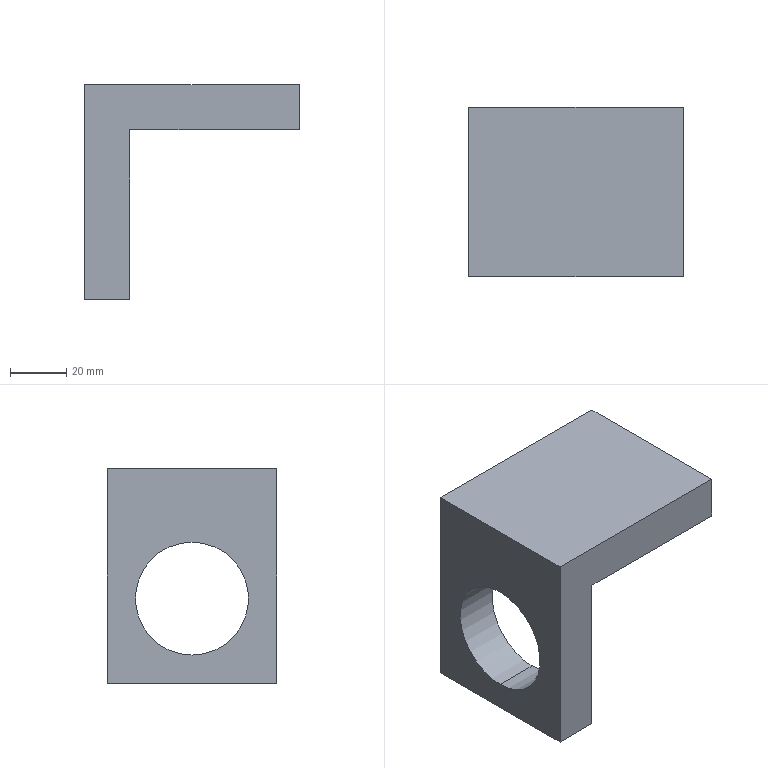Part | STEP file | PN_0009 Cylinder bracket | 1 solid | 10 faces | box 76 x 60 x 76 mm | volume 110454 mm3 | plane 8 | cylinder 2 | commonest cylinder face diameters 40 x2
STEP:
#1=CARTESIAN_POINT('',(0.,0.,0.));
#2=DIRECTION('',(0.,0.,1.));
#3=DIRECTION('',(1.,0.,0.));
#4=AXIS2_PLACEMENT_3D('',#1,#2,#3);
#5=CARTESIAN_POINT('',(-16.,30.,10.));
#6=VERTEX_POINT('',#5);
#7=CARTESIAN_POINT('',(0.,30.,10.));
#8=VERTEX_POINT('',#7);
#9=CARTESIAN_POINT('',(-80.,30.,10.));
#10=DIRECTION('',(1.,0.,0.));
#11=VECTOR('',#10,1.);
#12=LINE('',#9,#11);
#13=CARTESIAN_POINT('',(-80.,30.,30.));
#14=DIRECTION('',(1.,0.,0.));
#15=DIRECTION('',(0.,0.,-1.));
#16=AXIS2_PLACEMENT_3D('',#13,#14,#15);
#17=CYLINDRICAL_SURFACE('',#16,20.);
#18=CARTESIAN_POINT('',(6.283,0.));
#19=DIRECTION('',(0.,1.));
#20=VECTOR('',#19,1.);
#21=LINE('',#18,#20);
#22=(GEOMETRIC_REPRESENTATION_CONTEXT(2)PARAMETRIC_REPRESENTATION_CONTEXT()REPRESENTATION_CONTEXT('',''));
#23=DEFINITIONAL_REPRESENTATION('',(#21),#22);
#24=PCURVE('',#17,#23);
#25=CARTESIAN_POINT('',(-80.,30.,30.));
#26=DIRECTION('',(1.,0.,0.));
#27=DIRECTION('',(0.,0.,-1.));
#28=AXIS2_PLACEMENT_3D('',#25,#26,#27);
#29=CYLINDRICAL_SURFACE('',#28,20.);
#30=CARTESIAN_POINT('',(0.,0.));
#31=DIRECTION('',(0.,1.));
#32=VECTOR('',#31,1.);
#33=LINE('',#30,#32);
#34=(GEOMETRIC_REPRESENTATION_CONTEXT(2)PARAMETRIC_REPRESENTATION_CONTEXT()REPRESENTATION_CONTEXT('',''));
#35=DEFINITIONAL_REPRESENTATION('',(#33),#34);
#36=PCURVE('',#29,#35);
#37=SURFACE_CURVE('',#12,(#24,#36),.PCURVE_S1.);
#38=EDGE_CURVE('',#6,#8,#37,.T.);
#39=ORIENTED_EDGE('',*,*,#38,.T.);
#40=CARTESIAN_POINT('',(0.,30.,50.));
#41=VERTEX_POINT('',#40);
#42=CARTESIAN_POINT('',(0.,30.,30.));
#43=DIRECTION('',(1.,0.,0.));
#44=DIRECTION('',(0.,0.,-1.));
#45=AXIS2_PLACEMENT_3D('',#42,#43,#44);
#46=CIRCLE('',#45,20.);
#47=CARTESIAN_POINT('',(0.,80.));
#48=DIRECTION('',(1.,0.));
#49=VECTOR('',#48,1.);
#50=LINE('',#47,#49);
#51=(GEOMETRIC_REPRESENTATION_CONTEXT(2)PARAMETRIC_REPRESENTATION_CONTEXT()REPRESENTATION_CONTEXT('',''));
#52=DEFINITIONAL_REPRESENTATION('',(#50),#51);
#53=PCURVE('',#17,#52);
#54=CARTESIAN_POINT('',(0.,60.,0.));
#55=DIRECTION('',(-1.,0.,0.));
#56=DIRECTION('',(0.,0.,1.));
#57=AXIS2_PLACEMENT_3D('',#54,#55,#56);
#58=PLANE('',#57);
#59=CARTESIAN_POINT('',(10.,-30.));
#60=CARTESIAN_POINT('',(10.,4.641));
#61=CARTESIAN_POINT('',(40.,-12.679));
#62=CARTESIAN_POINT('',(70.,-30.));
#63=CARTESIAN_POINT('',(40.,-47.321));
#64=CARTESIAN_POINT('',(10.,-64.641));
#65=CARTESIAN_POINT('',(10.,-30.));
#66=(BOUNDED_CURVE()B_SPLINE_CURVE(2,(#59,#60,#61,#62,#63,#64,#65),.UNSPECIFIED.,.T.,.F.)B_SPLINE_CURVE_WITH_KNOTS((1,2,2,2,2,1),(-2.094,0.,2.094,4.189,6.283,8.378),.UNSPECIFIED.)CURVE()GEOMETRIC_REPRESENTATION_ITEM()RATIONAL_B_SPLINE_CURVE((1.,0.5,1.,0.5,1.,0.5,1.))REPRESENTATION_ITEM(''));
#67=(GEOMETRIC_REPRESENTATION_CONTEXT(2)PARAMETRIC_REPRESENTATION_CONTEXT()REPRESENTATION_CONTEXT('',''));
#68=DEFINITIONAL_REPRESENTATION('',(#66),#67);
#69=PCURVE('',#58,#68);
#70=SURFACE_CURVE('',#46,(#53,#69),.PCURVE_S1.);
#71=EDGE_CURVE('',#41,#8,#70,.T.);
#72=ORIENTED_EDGE('',*,*,#71,.F.);
#73=CARTESIAN_POINT('',(-16.,30.,50.));
#74=VERTEX_POINT('',#73);
#75=CARTESIAN_POINT('',(-80.,30.,50.));
#76=DIRECTION('',(1.,0.,0.));
#77=VECTOR('',#76,1.);
#78=LINE('',#75,#77);
#79=CARTESIAN_POINT('',(3.142,0.));
#80=DIRECTION('',(0.,1.));
#81=VECTOR('',#80,1.);
#82=LINE('',#79,#81);
#83=(GEOMETRIC_REPRESENTATION_CONTEXT(2)PARAMETRIC_REPRESENTATION_CONTEXT()REPRESENTATION_CONTEXT('',''));
#84=DEFINITIONAL_REPRESENTATION('',(#82),#83);
#85=PCURVE('',#17,#84);
#86=CARTESIAN_POINT('',(3.142,0.));
#87=DIRECTION('',(0.,1.));
#88=VECTOR('',#87,1.);
#89=LINE('',#86,#88);
#90=(GEOMETRIC_REPRESENTATION_CONTEXT(2)PARAMETRIC_REPRESENTATION_CONTEXT()REPRESENTATION_CONTEXT('',''));
#91=DEFINITIONAL_REPRESENTATION('',(#89),#90);
#92=PCURVE('',#29,#91);
#93=SURFACE_CURVE('',#78,(#85,#92),.PCURVE_S1.);
#94=EDGE_CURVE('',#74,#41,#93,.T.);
#95=ORIENTED_EDGE('',*,*,#94,.F.);
#96=CARTESIAN_POINT('',(-16.,30.,30.));
#97=DIRECTION('',(1.,0.,0.));
#98=DIRECTION('',(0.,0.,-1.));
#99=AXIS2_PLACEMENT_3D('',#96,#97,#98);
#100=CIRCLE('',#99,20.);
#101=CARTESIAN_POINT('',(0.,64.));
#102=DIRECTION('',(1.,0.));
#103=VECTOR('',#102,1.);
#104=LINE('',#101,#103);
#105=(GEOMETRIC_REPRESENTATION_CONTEXT(2)PARAMETRIC_REPRESENTATION_CONTEXT()REPRESENTATION_CONTEXT('',''));
#106=DEFINITIONAL_REPRESENTATION('',(#104),#105);
#107=PCURVE('',#17,#106);
#108=CARTESIAN_POINT('',(-16.,60.,0.));
#109=DIRECTION('',(1.,0.,0.));
#110=DIRECTION('',(0.,0.,-1.));
#111=AXIS2_PLACEMENT_3D('',#108,#109,#110);
#112=PLANE('',#111);
#113=CARTESIAN_POINT('',(-30.,-30.));
#114=DIRECTION('',(1.,0.));
#115=AXIS2_PLACEMENT_2D('',#113,#114);
#116=CIRCLE('',#115,20.);
#117=(GEOMETRIC_REPRESENTATION_CONTEXT(2)PARAMETRIC_REPRESENTATION_CONTEXT()REPRESENTATION_CONTEXT('',''));
#118=DEFINITIONAL_REPRESENTATION('',(#116),#117);
#119=PCURVE('',#112,#118);
#120=SURFACE_CURVE('',#100,(#107,#119),.PCURVE_S1.);
#121=EDGE_CURVE('',#74,#6,#120,.T.);
#122=ORIENTED_EDGE('',*,*,#121,.T.);
#123=EDGE_LOOP('',(#39,#72,#95,#122));
#124=FACE_BOUND('',#123,.F.);
#125=ADVANCED_FACE('',(#124),#17,.F.);
#126=CARTESIAN_POINT('',(0.,0.,0.));
#127=VERTEX_POINT('',#126);
#128=CARTESIAN_POINT('',(-16.,0.,0.));
#129=VERTEX_POINT('',#128);
#130=CARTESIAN_POINT('',(-16.,0.,0.));
#131=DIRECTION('',(-1.,0.,0.));
#132=VECTOR('',#131,1.);
#133=LINE('',#130,#132);
#134=CARTESIAN_POINT('',(-16.,60.,0.));
#135=DIRECTION('',(0.,0.,1.));
#136=DIRECTION('',(1.,0.,0.));
#137=AXIS2_PLACEMENT_3D('',#134,#135,#136);
#138=PLANE('',#137);
#139=CARTESIAN_POINT('',(0.,-60.));
#140=DIRECTION('',(-1.,0.));
#141=VECTOR('',#140,1.);
#142=LINE('',#139,#141);
#143=(GEOMETRIC_REPRESENTATION_CONTEXT(2)PARAMETRIC_REPRESENTATION_CONTEXT()REPRESENTATION_CONTEXT('',''));
#144=DEFINITIONAL_REPRESENTATION('',(#142),#143);
#145=PCURVE('',#138,#144);
#146=CARTESIAN_POINT('',(0.,0.,0.));
#147=DIRECTION('',(0.,-1.,0.));
#148=DIRECTION('',(0.,0.,-1.));
#149=AXIS2_PLACEMENT_3D('',#146,#147,#148);
#150=PLANE('',#149);
#151=CARTESIAN_POINT('',(0.,-16.));
#152=DIRECTION('',(0.,-1.));
#153=VECTOR('',#152,1.);
#154=LINE('',#151,#153);
#155=(GEOMETRIC_REPRESENTATION_CONTEXT(2)PARAMETRIC_REPRESENTATION_CONTEXT()REPRESENTATION_CONTEXT('',''));
#156=DEFINITIONAL_REPRESENTATION('',(#154),#155);
#157=PCURVE('',#150,#156);
#158=SURFACE_CURVE('',#133,(#145,#157),.PCURVE_S1.);
#159=EDGE_CURVE('',#127,#129,#158,.T.);
#160=ORIENTED_EDGE('',*,*,#159,.T.);
#161=CARTESIAN_POINT('',(-16.,60.,0.));
#162=VERTEX_POINT('',#161);
#163=CARTESIAN_POINT('',(-16.,60.,0.));
#164=DIRECTION('',(0.,-1.,0.));
#165=VECTOR('',#164,1.);
#166=LINE('',#163,#165);
#167=CARTESIAN_POINT('',(0.,0.));
#168=DIRECTION('',(0.,-1.));
#169=VECTOR('',#168,1.);
#170=LINE('',#167,#169);
#171=(GEOMETRIC_REPRESENTATION_CONTEXT(2)PARAMETRIC_REPRESENTATION_CONTEXT()REPRESENTATION_CONTEXT('',''));
#172=DEFINITIONAL_REPRESENTATION('',(#170),#171);
#173=PCURVE('',#138,#172);
#174=CARTESIAN_POINT('',(0.,0.));
#175=DIRECTION('',(0.,-1.));
#176=VECTOR('',#175,1.);
#177=LINE('',#174,#176);
#178=(GEOMETRIC_REPRESENTATION_CONTEXT(2)PARAMETRIC_REPRESENTATION_CONTEXT()REPRESENTATION_CONTEXT('',''));
#179=DEFINITIONAL_REPRESENTATION('',(#177),#178);
#180=PCURVE('',#112,#179);
#181=SURFACE_CURVE('',#166,(#173,#180),.PCURVE_S1.);
#182=EDGE_CURVE('',#162,#129,#181,.T.);
#183=ORIENTED_EDGE('',*,*,#182,.F.);
#184=CARTESIAN_POINT('',(0.,60.,0.));
#185=VERTEX_POINT('',#184);
#186=CARTESIAN_POINT('',(-16.,60.,0.));
#187=DIRECTION('',(-1.,0.,0.));
#188=VECTOR('',#187,1.);
#189=LINE('',#186,#188);
#190=CARTESIAN_POINT('',(0.,0.));
#191=DIRECTION('',(-1.,0.));
#192=VECTOR('',#191,1.);
#193=LINE('',#190,#192);
#194=(GEOMETRIC_REPRESENTATION_CONTEXT(2)PARAMETRIC_REPRESENTATION_CONTEXT()REPRESENTATION_CONTEXT('',''));
#195=DEFINITIONAL_REPRESENTATION('',(#193),#194);
#196=PCURVE('',#138,#195);
#197=CARTESIAN_POINT('',(0.,60.,0.));
#198=DIRECTION('',(0.,-1.,0.));
#199=DIRECTION('',(0.,0.,-1.));
#200=AXIS2_PLACEMENT_3D('',#197,#198,#199);
#201=PLANE('',#200);
#202=CARTESIAN_POINT('',(0.,-16.));
#203=DIRECTION('',(0.,-1.));
#204=VECTOR('',#203,1.);
#205=LINE('',#202,#204);
#206=(GEOMETRIC_REPRESENTATION_CONTEXT(2)PARAMETRIC_REPRESENTATION_CONTEXT()REPRESENTATION_CONTEXT('',''));
#207=DEFINITIONAL_REPRESENTATION('',(#205),#206);
#208=PCURVE('',#201,#207);
#209=SURFACE_CURVE('',#189,(#196,#208),.PCURVE_S1.);
#210=EDGE_CURVE('',#185,#162,#209,.T.);
#211=ORIENTED_EDGE('',*,*,#210,.F.);
#212=CARTESIAN_POINT('',(0.,60.,0.));
#213=DIRECTION('',(0.,-1.,0.));
#214=VECTOR('',#213,1.);
#215=LINE('',#212,#214);
#216=CARTESIAN_POINT('',(16.,0.));
#217=DIRECTION('',(0.,-1.));
#218=VECTOR('',#217,1.);
#219=LINE('',#216,#218);
#220=(GEOMETRIC_REPRESENTATION_CONTEXT(2)PARAMETRIC_REPRESENTATION_CONTEXT()REPRESENTATION_CONTEXT('',''));
#221=DEFINITIONAL_REPRESENTATION('',(#219),#220);
#222=PCURVE('',#138,#221);
#223=CARTESIAN_POINT('',(0.,0.));
#224=DIRECTION('',(0.,-1.));
#225=VECTOR('',#224,1.);
#226=LINE('',#223,#225);
#227=(GEOMETRIC_REPRESENTATION_CONTEXT(2)PARAMETRIC_REPRESENTATION_CONTEXT()REPRESENTATION_CONTEXT('',''));
#228=DEFINITIONAL_REPRESENTATION('',(#226),#227);
#229=PCURVE('',#58,#228);
#230=SURFACE_CURVE('',#215,(#222,#229),.PCURVE_S1.);
#231=EDGE_CURVE('',#185,#127,#230,.T.);
#232=ORIENTED_EDGE('',*,*,#231,.T.);
#233=EDGE_LOOP('',(#160,#183,#211,#232));
#234=FACE_BOUND('',#233,.T.);
#235=ADVANCED_FACE('',(#234),#138,.F.);
#236=CARTESIAN_POINT('',(-16.,30.,30.));
#237=DIRECTION('',(1.,0.,0.));
#238=DIRECTION('',(0.,0.,-1.));
#239=AXIS2_PLACEMENT_3D('',#236,#237,#238);
#240=CIRCLE('',#239,20.);
#241=CARTESIAN_POINT('',(-30.,-30.));
#242=DIRECTION('',(1.,0.));
#243=AXIS2_PLACEMENT_2D('',#241,#242);
#244=CIRCLE('',#243,20.);
#245=(GEOMETRIC_REPRESENTATION_CONTEXT(2)PARAMETRIC_REPRESENTATION_CONTEXT()REPRESENTATION_CONTEXT('',''));
#246=DEFINITIONAL_REPRESENTATION('',(#244),#245);
#247=PCURVE('',#112,#246);
#248=CARTESIAN_POINT('',(0.,64.));
#249=DIRECTION('',(1.,0.));
#250=VECTOR('',#249,1.);
#251=LINE('',#248,#250);
#252=(GEOMETRIC_REPRESENTATION_CONTEXT(2)PARAMETRIC_REPRESENTATION_CONTEXT()REPRESENTATION_CONTEXT('',''));
#253=DEFINITIONAL_REPRESENTATION('',(#251),#252);
#254=PCURVE('',#29,#253);
#255=SURFACE_CURVE('',#240,(#247,#254),.PCURVE_S1.);
#256=EDGE_CURVE('',#6,#74,#255,.T.);
#257=ORIENTED_EDGE('',*,*,#256,.T.);
#258=ORIENTED_EDGE('',*,*,#121,.T.);
#259=EDGE_LOOP('',(#257,#258));
#260=FACE_BOUND('',#259,.T.);
#261=CARTESIAN_POINT('',(-16.,0.,76.));
#262=VERTEX_POINT('',#261);
#263=CARTESIAN_POINT('',(-16.,0.,0.));
#264=DIRECTION('',(0.,0.,1.));
#265=VECTOR('',#264,1.);
#266=LINE('',#263,#265);
#267=CARTESIAN_POINT('',(0.,-60.));
#268=DIRECTION('',(-1.,0.));
#269=VECTOR('',#268,1.);
#270=LINE('',#267,#269);
#271=(GEOMETRIC_REPRESENTATION_CONTEXT(2)PARAMETRIC_REPRESENTATION_CONTEXT()REPRESENTATION_CONTEXT('',''));
#272=DEFINITIONAL_REPRESENTATION('',(#270),#271);
#273=PCURVE('',#112,#272);
#274=CARTESIAN_POINT('',(0.,-16.));
#275=DIRECTION('',(-1.,0.));
#276=VECTOR('',#275,1.);
#277=LINE('',#274,#276);
#278=(GEOMETRIC_REPRESENTATION_CONTEXT(2)PARAMETRIC_REPRESENTATION_CONTEXT()REPRESENTATION_CONTEXT('',''));
#279=DEFINITIONAL_REPRESENTATION('',(#277),#278);
#280=PCURVE('',#150,#279);
#281=SURFACE_CURVE('',#266,(#273,#280),.PCURVE_S1.);
#282=EDGE_CURVE('',#129,#262,#281,.T.);
#283=ORIENTED_EDGE('',*,*,#282,.T.);
#284=CARTESIAN_POINT('',(-16.,60.,76.));
#285=VERTEX_POINT('',#284);
#286=CARTESIAN_POINT('',(-16.,60.,76.));
#287=DIRECTION('',(0.,-1.,0.));
#288=VECTOR('',#287,1.);
#289=LINE('',#286,#288);
#290=CARTESIAN_POINT('',(-76.,0.));
#291=DIRECTION('',(0.,-1.));
#292=VECTOR('',#291,1.);
#293=LINE('',#290,#292);
#294=(GEOMETRIC_REPRESENTATION_CONTEXT(2)PARAMETRIC_REPRESENTATION_CONTEXT()REPRESENTATION_CONTEXT('',''));
#295=DEFINITIONAL_REPRESENTATION('',(#293),#294);
#296=PCURVE('',#112,#295);
#297=CARTESIAN_POINT('',(-16.,60.,76.));
#298=DIRECTION('',(0.,0.,-1.));
#299=DIRECTION('',(-1.,0.,0.));
#300=AXIS2_PLACEMENT_3D('',#297,#298,#299);
#301=PLANE('',#300);
#302=CARTESIAN_POINT('',(0.,0.));
#303=DIRECTION('',(0.,-1.));
#304=VECTOR('',#303,1.);
#305=LINE('',#302,#304);
#306=(GEOMETRIC_REPRESENTATION_CONTEXT(2)PARAMETRIC_REPRESENTATION_CONTEXT()REPRESENTATION_CONTEXT('',''));
#307=DEFINITIONAL_REPRESENTATION('',(#305),#306);
#308=PCURVE('',#301,#307);
#309=SURFACE_CURVE('',#289,(#296,#308),.PCURVE_S1.);
#310=EDGE_CURVE('',#285,#262,#309,.T.);
#311=ORIENTED_EDGE('',*,*,#310,.F.);
#312=CARTESIAN_POINT('',(-16.,60.,0.));
#313=DIRECTION('',(0.,0.,1.));
#314=VECTOR('',#313,1.);
#315=LINE('',#312,#314);
#316=CARTESIAN_POINT('',(0.,0.));
#317=DIRECTION('',(-1.,0.));
#318=VECTOR('',#317,1.);
#319=LINE('',#316,#318);
#320=(GEOMETRIC_REPRESENTATION_CONTEXT(2)PARAMETRIC_REPRESENTATION_CONTEXT()REPRESENTATION_CONTEXT('',''));
#321=DEFINITIONAL_REPRESENTATION('',(#319),#320);
#322=PCURVE('',#112,#321);
#323=CARTESIAN_POINT('',(0.,-16.));
#324=DIRECTION('',(-1.,0.));
#325=VECTOR('',#324,1.);
#326=LINE('',#323,#325);
#327=(GEOMETRIC_REPRESENTATION_CONTEXT(2)PARAMETRIC_REPRESENTATION_CONTEXT()REPRESENTATION_CONTEXT('',''));
#328=DEFINITIONAL_REPRESENTATION('',(#326),#327);
#329=PCURVE('',#201,#328);
#330=SURFACE_CURVE('',#315,(#322,#329),.PCURVE_S1.);
#331=EDGE_CURVE('',#162,#285,#330,.T.);
#332=ORIENTED_EDGE('',*,*,#331,.F.);
#333=ORIENTED_EDGE('',*,*,#182,.T.);
#334=EDGE_LOOP('',(#283,#311,#332,#333));
#335=FACE_BOUND('',#334,.T.);
#336=ADVANCED_FACE('',(#260,#335),#112,.F.);
#337=CARTESIAN_POINT('',(60.,0.,76.));
#338=VERTEX_POINT('',#337);
#339=CARTESIAN_POINT('',(-16.,0.,76.));
#340=DIRECTION('',(1.,0.,0.));
#341=VECTOR('',#340,1.);
#342=LINE('',#339,#341);
#343=CARTESIAN_POINT('',(0.,-60.));
#344=DIRECTION('',(-1.,0.));
#345=VECTOR('',#344,1.);
#346=LINE('',#343,#345);
#347=(GEOMETRIC_REPRESENTATION_CONTEXT(2)PARAMETRIC_REPRESENTATION_CONTEXT()REPRESENTATION_CONTEXT('',''));
#348=DEFINITIONAL_REPRESENTATION('',(#346),#347);
#349=PCURVE('',#301,#348);
#350=CARTESIAN_POINT('',(-76.,-16.));
#351=DIRECTION('',(0.,1.));
#352=VECTOR('',#351,1.);
#353=LINE('',#350,#352);
#354=(GEOMETRIC_REPRESENTATION_CONTEXT(2)PARAMETRIC_REPRESENTATION_CONTEXT()REPRESENTATION_CONTEXT('',''));
#355=DEFINITIONAL_REPRESENTATION('',(#353),#354);
#356=PCURVE('',#150,#355);
#357=SURFACE_CURVE('',#342,(#349,#356),.PCURVE_S1.);
#358=EDGE_CURVE('',#262,#338,#357,.T.);
#359=ORIENTED_EDGE('',*,*,#358,.T.);
#360=CARTESIAN_POINT('',(60.,60.,76.));
#361=VERTEX_POINT('',#360);
#362=CARTESIAN_POINT('',(60.,60.,76.));
#363=DIRECTION('',(0.,-1.,0.));
#364=VECTOR('',#363,1.);
#365=LINE('',#362,#364);
#366=CARTESIAN_POINT('',(-76.,0.));
#367=DIRECTION('',(0.,-1.));
#368=VECTOR('',#367,1.);
#369=LINE('',#366,#368);
#370=(GEOMETRIC_REPRESENTATION_CONTEXT(2)PARAMETRIC_REPRESENTATION_CONTEXT()REPRESENTATION_CONTEXT('',''));
#371=DEFINITIONAL_REPRESENTATION('',(#369),#370);
#372=PCURVE('',#301,#371);
#373=CARTESIAN_POINT('',(60.,60.,60.));
#374=DIRECTION('',(-1.,0.,0.));
#375=DIRECTION('',(0.,0.,1.));
#376=AXIS2_PLACEMENT_3D('',#373,#374,#375);
#377=PLANE('',#376);
#378=CARTESIAN_POINT('',(16.,0.));
#379=DIRECTION('',(0.,-1.));
#380=VECTOR('',#379,1.);
#381=LINE('',#378,#380);
#382=(GEOMETRIC_REPRESENTATION_CONTEXT(2)PARAMETRIC_REPRESENTATION_CONTEXT()REPRESENTATION_CONTEXT('',''));
#383=DEFINITIONAL_REPRESENTATION('',(#381),#382);
#384=PCURVE('',#377,#383);
#385=SURFACE_CURVE('',#365,(#372,#384),.PCURVE_S1.);
#386=EDGE_CURVE('',#361,#338,#385,.T.);
#387=ORIENTED_EDGE('',*,*,#386,.F.);
#388=CARTESIAN_POINT('',(-16.,60.,76.));
#389=DIRECTION('',(1.,0.,0.));
#390=VECTOR('',#389,1.);
#391=LINE('',#388,#390);
#392=CARTESIAN_POINT('',(0.,0.));
#393=DIRECTION('',(-1.,0.));
#394=VECTOR('',#393,1.);
#395=LINE('',#392,#394);
#396=(GEOMETRIC_REPRESENTATION_CONTEXT(2)PARAMETRIC_REPRESENTATION_CONTEXT()REPRESENTATION_CONTEXT('',''));
#397=DEFINITIONAL_REPRESENTATION('',(#395),#396);
#398=PCURVE('',#301,#397);
#399=CARTESIAN_POINT('',(-76.,-16.));
#400=DIRECTION('',(0.,1.));
#401=VECTOR('',#400,1.);
#402=LINE('',#399,#401);
#403=(GEOMETRIC_REPRESENTATION_CONTEXT(2)PARAMETRIC_REPRESENTATION_CONTEXT()REPRESENTATION_CONTEXT('',''));
#404=DEFINITIONAL_REPRESENTATION('',(#402),#403);
#405=PCURVE('',#201,#404);
#406=SURFACE_CURVE('',#391,(#398,#405),.PCURVE_S1.);
#407=EDGE_CURVE('',#285,#361,#406,.T.);
#408=ORIENTED_EDGE('',*,*,#407,.F.);
#409=ORIENTED_EDGE('',*,*,#310,.T.);
#410=EDGE_LOOP('',(#359,#387,#408,#409));
#411=FACE_BOUND('',#410,.T.);
#412=ADVANCED_FACE('',(#411),#301,.F.);
#413=CARTESIAN_POINT('',(60.,0.,60.));
#414=VERTEX_POINT('',#413);
#415=CARTESIAN_POINT('',(60.,0.,60.));
#416=DIRECTION('',(0.,0.,-1.));
#417=VECTOR('',#416,1.);
#418=LINE('',#415,#417);
#419=CARTESIAN_POINT('',(0.,-60.));
#420=DIRECTION('',(-1.,0.));
#421=VECTOR('',#420,1.);
#422=LINE('',#419,#421);
#423=(GEOMETRIC_REPRESENTATION_CONTEXT(2)PARAMETRIC_REPRESENTATION_CONTEXT()REPRESENTATION_CONTEXT('',''));
#424=DEFINITIONAL_REPRESENTATION('',(#422),#423);
#425=PCURVE('',#377,#424);
#426=CARTESIAN_POINT('',(-60.,60.));
#427=DIRECTION('',(1.,0.));
#428=VECTOR('',#427,1.);
#429=LINE('',#426,#428);
#430=(GEOMETRIC_REPRESENTATION_CONTEXT(2)PARAMETRIC_REPRESENTATION_CONTEXT()REPRESENTATION_CONTEXT('',''));
#431=DEFINITIONAL_REPRESENTATION('',(#429),#430);
#432=PCURVE('',#150,#431);
#433=SURFACE_CURVE('',#418,(#425,#432),.PCURVE_S1.);
#434=EDGE_CURVE('',#338,#414,#433,.T.);
#435=ORIENTED_EDGE('',*,*,#434,.T.);
#436=CARTESIAN_POINT('',(60.,60.,60.));
#437=VERTEX_POINT('',#436);
#438=CARTESIAN_POINT('',(60.,60.,60.));
#439=DIRECTION('',(0.,-1.,0.));
#440=VECTOR('',#439,1.);
#441=LINE('',#438,#440);
#442=CARTESIAN_POINT('',(0.,0.));
#443=DIRECTION('',(0.,-1.));
#444=VECTOR('',#443,1.);
#445=LINE('',#442,#444);
#446=(GEOMETRIC_REPRESENTATION_CONTEXT(2)PARAMETRIC_REPRESENTATION_CONTEXT()REPRESENTATION_CONTEXT('',''));
#447=DEFINITIONAL_REPRESENTATION('',(#445),#446);
#448=PCURVE('',#377,#447);
#449=CARTESIAN_POINT('',(0.,60.,60.));
#450=DIRECTION('',(0.,0.,1.));
#451=DIRECTION('',(1.,0.,0.));
#452=AXIS2_PLACEMENT_3D('',#449,#450,#451);
#453=PLANE('',#452);
#454=CARTESIAN_POINT('',(60.,0.));
#455=DIRECTION('',(0.,-1.));
#456=VECTOR('',#455,1.);
#457=LINE('',#454,#456);
#458=(GEOMETRIC_REPRESENTATION_CONTEXT(2)PARAMETRIC_REPRESENTATION_CONTEXT()REPRESENTATION_CONTEXT('',''));
#459=DEFINITIONAL_REPRESENTATION('',(#457),#458);
#460=PCURVE('',#453,#459);
#461=SURFACE_CURVE('',#441,(#448,#460),.PCURVE_S1.);
#462=EDGE_CURVE('',#437,#414,#461,.T.);
#463=ORIENTED_EDGE('',*,*,#462,.F.);
#464=CARTESIAN_POINT('',(60.,60.,60.));
#465=DIRECTION('',(0.,0.,-1.));
#466=VECTOR('',#465,1.);
#467=LINE('',#464,#466);
#468=CARTESIAN_POINT('',(0.,0.));
#469=DIRECTION('',(-1.,0.));
#470=VECTOR('',#469,1.);
#471=LINE('',#468,#470);
#472=(GEOMETRIC_REPRESENTATION_CONTEXT(2)PARAMETRIC_REPRESENTATION_CONTEXT()REPRESENTATION_CONTEXT('',''));
#473=DEFINITIONAL_REPRESENTATION('',(#471),#472);
#474=PCURVE('',#377,#473);
#475=CARTESIAN_POINT('',(-60.,60.));
#476=DIRECTION('',(1.,0.));
#477=VECTOR('',#476,1.);
#478=LINE('',#475,#477);
#479=(GEOMETRIC_REPRESENTATION_CONTEXT(2)PARAMETRIC_REPRESENTATION_CONTEXT()REPRESENTATION_CONTEXT('',''));
#480=DEFINITIONAL_REPRESENTATION('',(#478),#479);
#481=PCURVE('',#201,#480);
#482=SURFACE_CURVE('',#467,(#474,#481),.PCURVE_S1.);
#483=EDGE_CURVE('',#361,#437,#482,.T.);
#484=ORIENTED_EDGE('',*,*,#483,.F.);
#485=ORIENTED_EDGE('',*,*,#386,.T.);
#486=EDGE_LOOP('',(#435,#463,#484,#485));
#487=FACE_BOUND('',#486,.T.);
#488=ADVANCED_FACE('',(#487),#377,.F.);
#489=CARTESIAN_POINT('',(0.,0.,60.));
#490=VERTEX_POINT('',#489);
#491=CARTESIAN_POINT('',(0.,0.,60.));
#492=DIRECTION('',(-1.,0.,0.));
#493=VECTOR('',#492,1.);
#494=LINE('',#491,#493);
#495=CARTESIAN_POINT('',(0.,-60.));
#496=DIRECTION('',(-1.,0.));
#497=VECTOR('',#496,1.);
#498=LINE('',#495,#497);
#499=(GEOMETRIC_REPRESENTATION_CONTEXT(2)PARAMETRIC_REPRESENTATION_CONTEXT()REPRESENTATION_CONTEXT('',''));
#500=DEFINITIONAL_REPRESENTATION('',(#498),#499);
#501=PCURVE('',#453,#500);
#502=CARTESIAN_POINT('',(-60.,0.));
#503=DIRECTION('',(0.,-1.));
#504=VECTOR('',#503,1.);
#505=LINE('',#502,#504);
#506=(GEOMETRIC_REPRESENTATION_CONTEXT(2)PARAMETRIC_REPRESENTATION_CONTEXT()REPRESENTATION_CONTEXT('',''));
#507=DEFINITIONAL_REPRESENTATION('',(#505),#506);
#508=PCURVE('',#150,#507);
#509=SURFACE_CURVE('',#494,(#501,#508),.PCURVE_S1.);
#510=EDGE_CURVE('',#414,#490,#509,.T.);
#511=ORIENTED_EDGE('',*,*,#510,.T.);
#512=CARTESIAN_POINT('',(0.,60.,60.));
#513=VERTEX_POINT('',#512);
#514=CARTESIAN_POINT('',(0.,60.,60.));
#515=DIRECTION('',(0.,-1.,0.));
#516=VECTOR('',#515,1.);
#517=LINE('',#514,#516);
#518=CARTESIAN_POINT('',(0.,0.));
#519=DIRECTION('',(0.,-1.));
#520=VECTOR('',#519,1.);
#521=LINE('',#518,#520);
#522=(GEOMETRIC_REPRESENTATION_CONTEXT(2)PARAMETRIC_REPRESENTATION_CONTEXT()REPRESENTATION_CONTEXT('',''));
#523=DEFINITIONAL_REPRESENTATION('',(#521),#522);
#524=PCURVE('',#453,#523);
#525=CARTESIAN_POINT('',(60.,0.));
#526=DIRECTION('',(0.,-1.));
#527=VECTOR('',#526,1.);
#528=LINE('',#525,#527);
#529=(GEOMETRIC_REPRESENTATION_CONTEXT(2)PARAMETRIC_REPRESENTATION_CONTEXT()REPRESENTATION_CONTEXT('',''));
#530=DEFINITIONAL_REPRESENTATION('',(#528),#529);
#531=PCURVE('',#58,#530);
#532=SURFACE_CURVE('',#517,(#524,#531),.PCURVE_S1.);
#533=EDGE_CURVE('',#513,#490,#532,.T.);
#534=ORIENTED_EDGE('',*,*,#533,.F.);
#535=CARTESIAN_POINT('',(0.,60.,60.));
#536=DIRECTION('',(-1.,0.,0.));
#537=VECTOR('',#536,1.);
#538=LINE('',#535,#537);
#539=CARTESIAN_POINT('',(0.,0.));
#540=DIRECTION('',(-1.,0.));
#541=VECTOR('',#540,1.);
#542=LINE('',#539,#541);
#543=(GEOMETRIC_REPRESENTATION_CONTEXT(2)PARAMETRIC_REPRESENTATION_CONTEXT()REPRESENTATION_CONTEXT('',''));
#544=DEFINITIONAL_REPRESENTATION('',(#542),#543);
#545=PCURVE('',#453,#544);
#546=CARTESIAN_POINT('',(-60.,0.));
#547=DIRECTION('',(0.,-1.));
#548=VECTOR('',#547,1.);
#549=LINE('',#546,#548);
#550=(GEOMETRIC_REPRESENTATION_CONTEXT(2)PARAMETRIC_REPRESENTATION_CONTEXT()REPRESENTATION_CONTEXT('',''));
#551=DEFINITIONAL_REPRESENTATION('',(#549),#550);
#552=PCURVE('',#201,#551);
#553=SURFACE_CURVE('',#538,(#545,#552),.PCURVE_S1.);
#554=EDGE_CURVE('',#437,#513,#553,.T.);
#555=ORIENTED_EDGE('',*,*,#554,.F.);
#556=ORIENTED_EDGE('',*,*,#462,.T.);
#557=EDGE_LOOP('',(#511,#534,#555,#556));
#558=FACE_BOUND('',#557,.T.);
#559=ADVANCED_FACE('',(#558),#453,.F.);
#560=CARTESIAN_POINT('',(0.,30.,30.));
#561=DIRECTION('',(1.,0.,0.));
#562=DIRECTION('',(0.,0.,-1.));
#563=AXIS2_PLACEMENT_3D('',#560,#561,#562);
#564=CIRCLE('',#563,20.);
#565=CARTESIAN_POINT('',(10.,-30.));
#566=CARTESIAN_POINT('',(10.,4.641));
#567=CARTESIAN_POINT('',(40.,-12.679));
#568=CARTESIAN_POINT('',(70.,-30.));
#569=CARTESIAN_POINT('',(40.,-47.321));
#570=CARTESIAN_POINT('',(10.,-64.641));
#571=CARTESIAN_POINT('',(10.,-30.));
#572=(BOUNDED_CURVE()B_SPLINE_CURVE(2,(#565,#566,#567,#568,#569,#570,#571),.UNSPECIFIED.,.T.,.F.)B_SPLINE_CURVE_WITH_KNOTS((1,2,2,2,2,1),(-2.094,0.,2.094,4.189,6.283,8.378),.UNSPECIFIED.)CURVE()GEOMETRIC_REPRESENTATION_ITEM()RATIONAL_B_SPLINE_CURVE((1.,0.5,1.,0.5,1.,0.5,1.))REPRESENTATION_ITEM(''));
#573=(GEOMETRIC_REPRESENTATION_CONTEXT(2)PARAMETRIC_REPRESENTATION_CONTEXT()REPRESENTATION_CONTEXT('',''));
#574=DEFINITIONAL_REPRESENTATION('',(#572),#573);
#575=PCURVE('',#58,#574);
#576=CARTESIAN_POINT('',(0.,80.));
#577=DIRECTION('',(1.,0.));
#578=VECTOR('',#577,1.);
#579=LINE('',#576,#578);
#580=(GEOMETRIC_REPRESENTATION_CONTEXT(2)PARAMETRIC_REPRESENTATION_CONTEXT()REPRESENTATION_CONTEXT('',''));
#581=DEFINITIONAL_REPRESENTATION('',(#579),#580);
#582=PCURVE('',#29,#581);
#583=SURFACE_CURVE('',#564,(#575,#582),.PCURVE_S1.);
#584=EDGE_CURVE('',#8,#41,#583,.T.);
#585=ORIENTED_EDGE('',*,*,#584,.F.);
#586=ORIENTED_EDGE('',*,*,#71,.F.);
#587=EDGE_LOOP('',(#585,#586));
#588=FACE_BOUND('',#587,.T.);
#589=CARTESIAN_POINT('',(0.,0.,0.));
#590=DIRECTION('',(0.,0.,-1.));
#591=VECTOR('',#590,1.);
#592=LINE('',#589,#591);
#593=CARTESIAN_POINT('',(0.,-60.));
#594=DIRECTION('',(-1.,0.));
#595=VECTOR('',#594,1.);
#596=LINE('',#593,#595);
#597=(GEOMETRIC_REPRESENTATION_CONTEXT(2)PARAMETRIC_REPRESENTATION_CONTEXT()REPRESENTATION_CONTEXT('',''));
#598=DEFINITIONAL_REPRESENTATION('',(#596),#597);
#599=PCURVE('',#58,#598);
#600=CARTESIAN_POINT('',(0.,0.));
#601=DIRECTION('',(1.,0.));
#602=VECTOR('',#601,1.);
#603=LINE('',#600,#602);
#604=(GEOMETRIC_REPRESENTATION_CONTEXT(2)PARAMETRIC_REPRESENTATION_CONTEXT()REPRESENTATION_CONTEXT('',''));
#605=DEFINITIONAL_REPRESENTATION('',(#603),#604);
#606=PCURVE('',#150,#605);
#607=SURFACE_CURVE('',#592,(#599,#606),.PCURVE_S1.);
#608=EDGE_CURVE('',#490,#127,#607,.T.);
#609=ORIENTED_EDGE('',*,*,#608,.T.);
#610=ORIENTED_EDGE('',*,*,#231,.F.);
#611=CARTESIAN_POINT('',(0.,60.,0.));
#612=DIRECTION('',(0.,0.,-1.));
#613=VECTOR('',#612,1.);
#614=LINE('',#611,#613);
#615=CARTESIAN_POINT('',(0.,0.));
#616=DIRECTION('',(-1.,0.));
#617=VECTOR('',#616,1.);
#618=LINE('',#615,#617);
#619=(GEOMETRIC_REPRESENTATION_CONTEXT(2)PARAMETRIC_REPRESENTATION_CONTEXT()REPRESENTATION_CONTEXT('',''));
#620=DEFINITIONAL_REPRESENTATION('',(#618),#619);
#621=PCURVE('',#58,#620);
#622=CARTESIAN_POINT('',(0.,0.));
#623=DIRECTION('',(1.,0.));
#624=VECTOR('',#623,1.);
#625=LINE('',#622,#624);
#626=(GEOMETRIC_REPRESENTATION_CONTEXT(2)PARAMETRIC_REPRESENTATION_CONTEXT()REPRESENTATION_CONTEXT('',''));
#627=DEFINITIONAL_REPRESENTATION('',(#625),#626);
#628=PCURVE('',#201,#627);
#629=SURFACE_CURVE('',#614,(#621,#628),.PCURVE_S1.);
#630=EDGE_CURVE('',#513,#185,#629,.T.);
#631=ORIENTED_EDGE('',*,*,#630,.F.);
#632=ORIENTED_EDGE('',*,*,#533,.T.);
#633=EDGE_LOOP('',(#609,#610,#631,#632));
#634=FACE_BOUND('',#633,.T.);
#635=ADVANCED_FACE('',(#588,#634),#58,.F.);
#636=ORIENTED_EDGE('',*,*,#210,.T.);
#637=ORIENTED_EDGE('',*,*,#331,.T.);
#638=ORIENTED_EDGE('',*,*,#407,.T.);
#639=ORIENTED_EDGE('',*,*,#483,.T.);
#640=ORIENTED_EDGE('',*,*,#554,.T.);
#641=ORIENTED_EDGE('',*,*,#630,.T.);
#642=EDGE_LOOP('',(#636,#637,#638,#639,#640,#641));
#643=FACE_BOUND('',#642,.T.);
#644=ADVANCED_FACE('',(#643),#201,.F.);
#645=ORIENTED_EDGE('',*,*,#159,.F.);
#646=ORIENTED_EDGE('',*,*,#608,.F.);
#647=ORIENTED_EDGE('',*,*,#510,.F.);
#648=ORIENTED_EDGE('',*,*,#434,.F.);
#649=ORIENTED_EDGE('',*,*,#358,.F.);
#650=ORIENTED_EDGE('',*,*,#282,.F.);
#651=EDGE_LOOP('',(#645,#646,#647,#648,#649,#650));
#652=FACE_BOUND('',#651,.T.);
#653=ADVANCED_FACE('',(#652),#150,.T.);
#654=ORIENTED_EDGE('',*,*,#584,.F.);
#655=ORIENTED_EDGE('',*,*,#38,.F.);
#656=ORIENTED_EDGE('',*,*,#256,.T.);
#657=ORIENTED_EDGE('',*,*,#94,.T.);
#658=EDGE_LOOP('',(#654,#655,#656,#657));
#659=FACE_BOUND('',#658,.F.);
#660=ADVANCED_FACE('',(#659),#29,.F.);
#661=CLOSED_SHELL('',(#125,#235,#336,#412,#488,#559,#635,#644,#653,#660));
#662=MANIFOLD_SOLID_BREP('',#661);
#663=(LENGTH_UNIT()NAMED_UNIT(*)SI_UNIT(.MILLI.,.METRE.));
#664=UNCERTAINTY_MEASURE_WITH_UNIT(LENGTH_MEASURE(0.0000001),#663,'','');
#665=(NAMED_UNIT(*)PLANE_ANGLE_UNIT()SI_UNIT($,.RADIAN.));
#666=(NAMED_UNIT(*)SI_UNIT($,.STERADIAN.)SOLID_ANGLE_UNIT());
#667=(GEOMETRIC_REPRESENTATION_CONTEXT(3)GLOBAL_UNCERTAINTY_ASSIGNED_CONTEXT((#664))GLOBAL_UNIT_ASSIGNED_CONTEXT((#663,#665,#666))REPRESENTATION_CONTEXT('',''));
#668=ADVANCED_BREP_SHAPE_REPRESENTATION('',(#4,#662),#667);